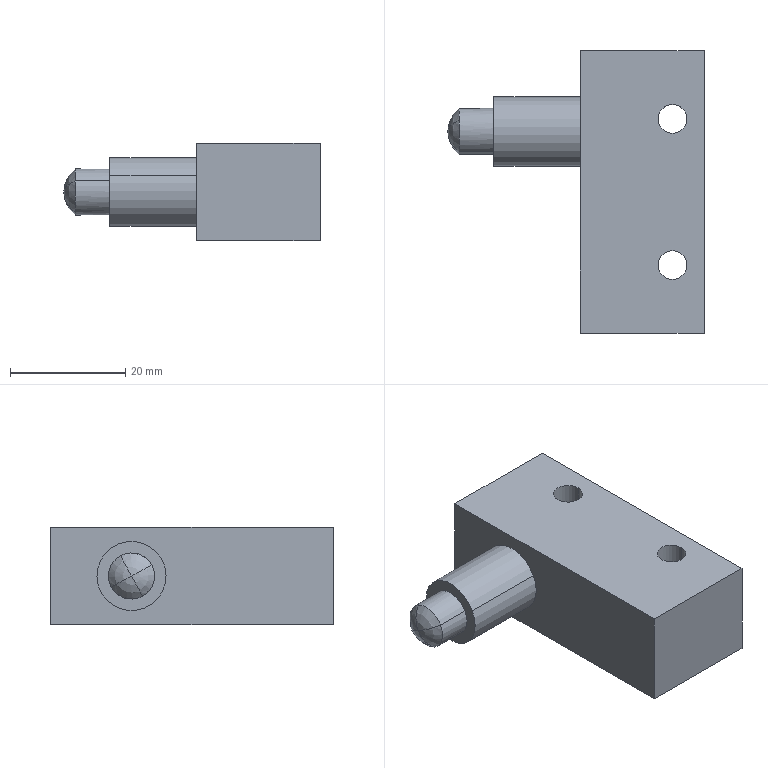Part | CATIA | 1 solid | 19 faces | box 44.5 x 49 x 17 mm | volume 19294 mm3 | cylinder 8 | plane 7 | sphere 4 | commonest cylinder face diameters 5 x4 8 x2 12 x2
STEP:
#1=CARTESIAN_POINT('',(-16.,17.935,11.377));
#2=VERTEX_POINT('',#1);
#3=CARTESIAN_POINT('',(-31.,17.935,11.377));
#4=VERTEX_POINT('',#3);
#5=CARTESIAN_POINT('',(-27.5,17.935,11.377));
#6=DIRECTION('',(-1.,0.,0.));
#7=VECTOR('',#6,1.);
#8=LINE('',#5,#7);
#9=EDGE_CURVE('',#2,#4,#8,.T.);
#10=ORIENTED_EDGE('',*,*,#9,.T.);
#11=CARTESIAN_POINT('',(-31.,28.465,5.623));
#12=VERTEX_POINT('',#11);
#13=CARTESIAN_POINT('',(-31.,23.2,8.5));
#14=DIRECTION('',(-1.,0.,0.));
#15=AXIS2_PLACEMENT_3D('',#13,#14,$);
#16=CIRCLE('',#15,6.);
#17=EDGE_CURVE('',#12,#4,#16,.T.);
#18=ORIENTED_EDGE('',*,*,#17,.F.);
#19=CARTESIAN_POINT('',(-16.,28.465,5.623));
#20=VERTEX_POINT('',#19);
#21=CARTESIAN_POINT('',(-27.5,28.465,5.623));
#22=DIRECTION('',(-1.,0.,0.));
#23=VECTOR('',#22,1.);
#24=LINE('',#21,#23);
#25=EDGE_CURVE('',#20,#12,#24,.T.);
#26=ORIENTED_EDGE('',*,*,#25,.F.);
#27=CARTESIAN_POINT('',(-16.,23.2,8.5));
#28=DIRECTION('',(-1.,0.,0.));
#29=AXIS2_PLACEMENT_3D('',#27,#28,$);
#30=CIRCLE('',#29,6.);
#31=EDGE_CURVE('',#20,#2,#30,.T.);
#32=ORIENTED_EDGE('',*,*,#31,.T.);
#33=EDGE_LOOP('',(#10,#18,#26,#32));
#34=FACE_OUTER_BOUND('',#33,.T.);
#35=CARTESIAN_POINT('',(-27.5,23.2,8.5));
#36=DIRECTION('',(-1.,0.,0.));
#37=DIRECTION('',(0.,0.8776,-0.4794));
#38=AXIS2_PLACEMENT_3D('',#35,#36,#37);
#39=CYLINDRICAL_SURFACE('',#38,6.);
#40=ADVANCED_FACE('',(#34),#39,.T.);
#41=ORIENTED_EDGE('',*,*,#25,.T.);
#42=CARTESIAN_POINT('',(-31.,23.2,8.5));
#43=DIRECTION('',(-1.,0.,0.));
#44=AXIS2_PLACEMENT_3D('',#42,#43,$);
#45=CIRCLE('',#44,6.);
#46=EDGE_CURVE('',#4,#12,#45,.T.);
#47=ORIENTED_EDGE('',*,*,#46,.F.);
#48=ORIENTED_EDGE('',*,*,#9,.F.);
#49=CARTESIAN_POINT('',(-16.,23.2,8.5));
#50=DIRECTION('',(-1.,0.,0.));
#51=AXIS2_PLACEMENT_3D('',#49,#50,$);
#52=CIRCLE('',#51,6.);
#53=EDGE_CURVE('',#2,#20,#52,.T.);
#54=ORIENTED_EDGE('',*,*,#53,.T.);
#55=EDGE_LOOP('',(#41,#47,#48,#54));
#56=FACE_OUTER_BOUND('',#55,.T.);
#57=CARTESIAN_POINT('',(-27.5,23.2,8.5));
#58=DIRECTION('',(-1.,0.,0.));
#59=DIRECTION('',(0.,-0.8776,0.4794));
#60=AXIS2_PLACEMENT_3D('',#57,#58,#59);
#61=CYLINDRICAL_SURFACE('',#60,6.);
#62=ADVANCED_FACE('',(#56),#61,.T.);
#63=ORIENTED_EDGE('',*,*,#46,.T.);
#64=ORIENTED_EDGE('',*,*,#17,.T.);
#65=EDGE_LOOP('',(#63,#64));
#66=FACE_OUTER_BOUND('',#65,.T.);
#67=CARTESIAN_POINT('',(-31.,26.71,6.582));
#68=VERTEX_POINT('',#67);
#69=CARTESIAN_POINT('',(-31.,19.69,10.418));
#70=VERTEX_POINT('',#69);
#71=CARTESIAN_POINT('',(-31.,23.2,8.5));
#72=DIRECTION('',(-1.,0.,0.));
#73=AXIS2_PLACEMENT_3D('',#71,#72,$);
#74=CIRCLE('',#73,4.);
#75=EDGE_CURVE('',#68,#70,#74,.T.);
#76=ORIENTED_EDGE('',*,*,#75,.F.);
#77=CARTESIAN_POINT('',(-31.,23.2,8.5));
#78=DIRECTION('',(-1.,0.,0.));
#79=AXIS2_PLACEMENT_3D('',#77,#78,$);
#80=CIRCLE('',#79,4.);
#81=EDGE_CURVE('',#70,#68,#80,.T.);
#82=ORIENTED_EDGE('',*,*,#81,.F.);
#83=EDGE_LOOP('',(#76,#82));
#84=FACE_BOUND('',#83,.T.);
#85=CARTESIAN_POINT('',(-31.,29.2,8.5));
#86=DIRECTION('',(-1.,0.,0.));
#87=DIRECTION('',(0.,1.,0.));
#88=AXIS2_PLACEMENT_3D('',#85,#86,#87);
#89=PLANE('',#88);
#90=ADVANCED_FACE('',(#66,#84),#89,.T.);
#91=CARTESIAN_POINT('',(-16.,37.2,0.));
#92=VERTEX_POINT('',#91);
#93=CARTESIAN_POINT('',(-16.,37.2,17.));
#94=VERTEX_POINT('',#93);
#95=CARTESIAN_POINT('',(-16.,37.2,8.5));
#96=DIRECTION('',(0.,0.,1.));
#97=VECTOR('',#96,1.);
#98=LINE('',#95,#97);
#99=EDGE_CURVE('',#92,#94,#98,.T.);
#100=ORIENTED_EDGE('',*,*,#99,.F.);
#101=CARTESIAN_POINT('',(-16.,-11.8,0.));
#102=VERTEX_POINT('',#101);
#103=CARTESIAN_POINT('',(-16.,12.7,0.));
#104=DIRECTION('',(0.,-1.,0.));
#105=VECTOR('',#104,1.);
#106=LINE('',#103,#105);
#107=EDGE_CURVE('',#92,#102,#106,.T.);
#108=ORIENTED_EDGE('',*,*,#107,.T.);
#109=CARTESIAN_POINT('',(-16.,-11.8,17.));
#110=VERTEX_POINT('',#109);
#111=CARTESIAN_POINT('',(-16.,-11.8,8.5));
#112=DIRECTION('',(0.,0.,1.));
#113=VECTOR('',#112,1.);
#114=LINE('',#111,#113);
#115=EDGE_CURVE('',#102,#110,#114,.T.);
#116=ORIENTED_EDGE('',*,*,#115,.T.);
#117=CARTESIAN_POINT('',(-16.,12.7,17.));
#118=DIRECTION('',(0.,-1.,0.));
#119=VECTOR('',#118,1.);
#120=LINE('',#117,#119);
#121=EDGE_CURVE('',#94,#110,#120,.T.);
#122=ORIENTED_EDGE('',*,*,#121,.F.);
#123=EDGE_LOOP('',(#100,#108,#116,#122));
#124=FACE_OUTER_BOUND('',#123,.T.);
#125=ORIENTED_EDGE('',*,*,#31,.F.);
#126=ORIENTED_EDGE('',*,*,#53,.F.);
#127=EDGE_LOOP('',(#125,#126));
#128=FACE_BOUND('',#127,.T.);
#129=CARTESIAN_POINT('',(-16.,37.2,0.));
#130=DIRECTION('',(-1.,0.,0.));
#131=DIRECTION('',(0.,-1.,0.));
#132=AXIS2_PLACEMENT_3D('',#129,#130,#131);
#133=PLANE('',#132);
#134=ADVANCED_FACE('',(#124,#128),#133,.T.);
#135=CARTESIAN_POINT('',(-37.,19.69,10.418));
#136=VERTEX_POINT('',#135);
#137=CARTESIAN_POINT('',(-27.5,19.69,10.418));
#138=DIRECTION('',(-1.,0.,0.));
#139=VECTOR('',#138,1.);
#140=LINE('',#137,#139);
#141=EDGE_CURVE('',#70,#136,#140,.T.);
#142=ORIENTED_EDGE('',*,*,#141,.T.);
#143=CARTESIAN_POINT('',(-37.,21.282,4.99));
#144=VERTEX_POINT('',#143);
#145=CARTESIAN_POINT('',(-37.,23.2,8.5));
#146=DIRECTION('',(-1.,0.,0.));
#147=AXIS2_PLACEMENT_3D('',#145,#146,$);
#148=CIRCLE('',#147,4.);
#149=EDGE_CURVE('',#144,#136,#148,.T.);
#150=ORIENTED_EDGE('',*,*,#149,.F.);
#151=CARTESIAN_POINT('',(-37.,26.71,6.582));
#152=VERTEX_POINT('',#151);
#153=CARTESIAN_POINT('',(-37.,23.2,8.5));
#154=DIRECTION('',(-1.,0.,0.));
#155=AXIS2_PLACEMENT_3D('',#153,#154,$);
#156=CIRCLE('',#155,4.);
#157=EDGE_CURVE('',#152,#144,#156,.T.);
#158=ORIENTED_EDGE('',*,*,#157,.F.);
#159=CARTESIAN_POINT('',(-27.5,26.71,6.582));
#160=DIRECTION('',(-1.,0.,0.));
#161=VECTOR('',#160,1.);
#162=LINE('',#159,#161);
#163=EDGE_CURVE('',#68,#152,#162,.T.);
#164=ORIENTED_EDGE('',*,*,#163,.F.);
#165=ORIENTED_EDGE('',*,*,#75,.T.);
#166=EDGE_LOOP('',(#142,#150,#158,#164,#165));
#167=FACE_OUTER_BOUND('',#166,.T.);
#168=CARTESIAN_POINT('',(-27.5,23.2,8.5));
#169=DIRECTION('',(-1.,0.,0.));
#170=DIRECTION('',(0.,0.8776,-0.4794));
#171=AXIS2_PLACEMENT_3D('',#168,#169,#170);
#172=CYLINDRICAL_SURFACE('',#171,4.);
#173=ADVANCED_FACE('',(#167),#172,.T.);
#174=ORIENTED_EDGE('',*,*,#163,.T.);
#175=CARTESIAN_POINT('',(-37.,25.118,12.01));
#176=VERTEX_POINT('',#175);
#177=CARTESIAN_POINT('',(-37.,23.2,8.5));
#178=DIRECTION('',(-1.,0.,0.));
#179=AXIS2_PLACEMENT_3D('',#177,#178,$);
#180=CIRCLE('',#179,4.);
#181=EDGE_CURVE('',#176,#152,#180,.T.);
#182=ORIENTED_EDGE('',*,*,#181,.F.);
#183=CARTESIAN_POINT('',(-37.,23.2,8.5));
#184=DIRECTION('',(-1.,0.,0.));
#185=AXIS2_PLACEMENT_3D('',#183,#184,$);
#186=CIRCLE('',#185,4.);
#187=EDGE_CURVE('',#136,#176,#186,.T.);
#188=ORIENTED_EDGE('',*,*,#187,.F.);
#189=ORIENTED_EDGE('',*,*,#141,.F.);
#190=ORIENTED_EDGE('',*,*,#81,.T.);
#191=EDGE_LOOP('',(#174,#182,#188,#189,#190));
#192=FACE_OUTER_BOUND('',#191,.T.);
#193=CARTESIAN_POINT('',(-27.5,23.2,8.5));
#194=DIRECTION('',(-1.,0.,0.));
#195=DIRECTION('',(0.,-0.8776,0.4794));
#196=AXIS2_PLACEMENT_3D('',#193,#194,#195);
#197=CYLINDRICAL_SURFACE('',#196,4.);
#198=ADVANCED_FACE('',(#192),#197,.T.);
#199=CARTESIAN_POINT('',(5.5,37.2,0.));
#200=VERTEX_POINT('',#199);
#201=CARTESIAN_POINT('',(5.5,37.2,17.));
#202=VERTEX_POINT('',#201);
#203=CARTESIAN_POINT('',(5.5,37.2,8.5));
#204=DIRECTION('',(0.,0.,1.));
#205=VECTOR('',#204,1.);
#206=LINE('',#203,#205);
#207=EDGE_CURVE('',#200,#202,#206,.T.);
#208=ORIENTED_EDGE('',*,*,#207,.F.);
#209=CARTESIAN_POINT('',(-5.25,37.2,0.));
#210=DIRECTION('',(1.,0.,0.));
#211=VECTOR('',#210,1.);
#212=LINE('',#209,#211);
#213=EDGE_CURVE('',#200,#92,#212,.F.);
#214=ORIENTED_EDGE('',*,*,#213,.T.);
#215=ORIENTED_EDGE('',*,*,#99,.T.);
#216=CARTESIAN_POINT('',(-5.25,37.2,17.));
#217=DIRECTION('',(1.,0.,0.));
#218=VECTOR('',#217,1.);
#219=LINE('',#216,#218);
#220=EDGE_CURVE('',#202,#94,#219,.F.);
#221=ORIENTED_EDGE('',*,*,#220,.F.);
#222=EDGE_LOOP('',(#208,#214,#215,#221));
#223=FACE_OUTER_BOUND('',#222,.T.);
#224=CARTESIAN_POINT('',(-16.,37.2,0.));
#225=DIRECTION('',(0.,-1.,0.));
#226=DIRECTION('',(1.,0.,0.));
#227=AXIS2_PLACEMENT_3D('',#224,#225,#226);
#228=PLANE('',#227);
#229=ADVANCED_FACE('',(#223),#228,.F.);
#230=ORIENTED_EDGE('',*,*,#213,.F.);
#231=CARTESIAN_POINT('',(5.5,-11.8,0.));
#232=VERTEX_POINT('',#231);
#233=CARTESIAN_POINT('',(5.5,12.7,0.));
#234=DIRECTION('',(0.,1.,0.));
#235=VECTOR('',#234,1.);
#236=LINE('',#233,#235);
#237=EDGE_CURVE('',#232,#200,#236,.T.);
#238=ORIENTED_EDGE('',*,*,#237,.F.);
#239=CARTESIAN_POINT('',(-5.25,-11.8,0.));
#240=DIRECTION('',(-1.,0.,0.));
#241=VECTOR('',#240,1.);
#242=LINE('',#239,#241);
#243=EDGE_CURVE('',#102,#232,#242,.F.);
#244=ORIENTED_EDGE('',*,*,#243,.F.);
#245=ORIENTED_EDGE('',*,*,#107,.F.);
#246=EDGE_LOOP('',(#230,#238,#244,#245));
#247=FACE_OUTER_BOUND('',#246,.T.);
#248=CARTESIAN_POINT('',(2.5,25.4,0.));
#249=VERTEX_POINT('',#248);
#250=CARTESIAN_POINT('',(-2.5,25.4,0.));
#251=VERTEX_POINT('',#250);
#252=CARTESIAN_POINT('',(0.,25.4,0.));
#253=DIRECTION('',(0.,0.,1.));
#254=AXIS2_PLACEMENT_3D('',#252,#253,$);
#255=CIRCLE('',#254,2.5);
#256=EDGE_CURVE('',#249,#251,#255,.T.);
#257=ORIENTED_EDGE('',*,*,#256,.T.);
#258=CARTESIAN_POINT('',(0.,25.4,0.));
#259=DIRECTION('',(0.,0.,1.));
#260=AXIS2_PLACEMENT_3D('',#258,#259,$);
#261=CIRCLE('',#260,2.5);
#262=EDGE_CURVE('',#251,#249,#261,.T.);
#263=ORIENTED_EDGE('',*,*,#262,.T.);
#264=EDGE_LOOP('',(#257,#263));
#265=FACE_BOUND('',#264,.T.);
#266=CARTESIAN_POINT('',(2.5,0.,0.));
#267=VERTEX_POINT('',#266);
#268=CARTESIAN_POINT('',(-2.5,0.,0.));
#269=VERTEX_POINT('',#268);
#270=CARTESIAN_POINT('',(0.,0.,0.));
#271=DIRECTION('',(0.,0.,1.));
#272=AXIS2_PLACEMENT_3D('',#270,#271,$);
#273=CIRCLE('',#272,2.5);
#274=EDGE_CURVE('',#267,#269,#273,.T.);
#275=ORIENTED_EDGE('',*,*,#274,.T.);
#276=CARTESIAN_POINT('',(0.,0.,0.));
#277=DIRECTION('',(0.,0.,1.));
#278=AXIS2_PLACEMENT_3D('',#276,#277,$);
#279=CIRCLE('',#278,2.5);
#280=EDGE_CURVE('',#269,#267,#279,.T.);
#281=ORIENTED_EDGE('',*,*,#280,.T.);
#282=EDGE_LOOP('',(#275,#281));
#283=FACE_BOUND('',#282,.T.);
#284=CARTESIAN_POINT('',(0.,0.,0.));
#285=DIRECTION('',(0.,0.,1.));
#286=DIRECTION('',(1.,0.,0.));
#287=AXIS2_PLACEMENT_3D('',#284,#285,#286);
#288=PLANE('',#287);
#289=ADVANCED_FACE('',(#247,#265,#283),#288,.F.);
#290=ORIENTED_EDGE('',*,*,#115,.F.);
#291=ORIENTED_EDGE('',*,*,#243,.T.);
#292=CARTESIAN_POINT('',(5.5,-11.8,17.));
#293=VERTEX_POINT('',#292);
#294=CARTESIAN_POINT('',(5.5,-11.8,8.5));
#295=DIRECTION('',(0.,0.,1.));
#296=VECTOR('',#295,1.);
#297=LINE('',#294,#296);
#298=EDGE_CURVE('',#232,#293,#297,.T.);
#299=ORIENTED_EDGE('',*,*,#298,.T.);
#300=CARTESIAN_POINT('',(-5.25,-11.8,17.));
#301=DIRECTION('',(-1.,0.,0.));
#302=VECTOR('',#301,1.);
#303=LINE('',#300,#302);
#304=EDGE_CURVE('',#110,#293,#303,.F.);
#305=ORIENTED_EDGE('',*,*,#304,.F.);
#306=EDGE_LOOP('',(#290,#291,#299,#305));
#307=FACE_OUTER_BOUND('',#306,.T.);
#308=CARTESIAN_POINT('',(5.5,-11.8,0.));
#309=DIRECTION('',(0.,1.,0.));
#310=DIRECTION('',(-1.,0.,0.));
#311=AXIS2_PLACEMENT_3D('',#308,#309,#310);
#312=PLANE('',#311);
#313=ADVANCED_FACE('',(#307),#312,.F.);
#314=ORIENTED_EDGE('',*,*,#121,.T.);
#315=ORIENTED_EDGE('',*,*,#304,.T.);
#316=CARTESIAN_POINT('',(5.5,12.7,17.));
#317=DIRECTION('',(0.,1.,0.));
#318=VECTOR('',#317,1.);
#319=LINE('',#316,#318);
#320=EDGE_CURVE('',#293,#202,#319,.T.);
#321=ORIENTED_EDGE('',*,*,#320,.T.);
#322=ORIENTED_EDGE('',*,*,#220,.T.);
#323=EDGE_LOOP('',(#314,#315,#321,#322));
#324=FACE_OUTER_BOUND('',#323,.T.);
#325=CARTESIAN_POINT('',(2.5,25.4,17.));
#326=VERTEX_POINT('',#325);
#327=CARTESIAN_POINT('',(-2.5,25.4,17.));
#328=VERTEX_POINT('',#327);
#329=CARTESIAN_POINT('',(0.,25.4,17.));
#330=DIRECTION('',(0.,0.,1.));
#331=AXIS2_PLACEMENT_3D('',#329,#330,$);
#332=CIRCLE('',#331,2.5);
#333=EDGE_CURVE('',#326,#328,#332,.T.);
#334=ORIENTED_EDGE('',*,*,#333,.F.);
#335=CARTESIAN_POINT('',(0.,25.4,17.));
#336=DIRECTION('',(0.,0.,1.));
#337=AXIS2_PLACEMENT_3D('',#335,#336,$);
#338=CIRCLE('',#337,2.5);
#339=EDGE_CURVE('',#328,#326,#338,.T.);
#340=ORIENTED_EDGE('',*,*,#339,.F.);
#341=EDGE_LOOP('',(#334,#340));
#342=FACE_BOUND('',#341,.T.);
#343=CARTESIAN_POINT('',(2.5,0.,17.));
#344=VERTEX_POINT('',#343);
#345=CARTESIAN_POINT('',(-2.5,0.,17.));
#346=VERTEX_POINT('',#345);
#347=CARTESIAN_POINT('',(0.,0.,17.));
#348=DIRECTION('',(0.,0.,1.));
#349=AXIS2_PLACEMENT_3D('',#347,#348,$);
#350=CIRCLE('',#349,2.5);
#351=EDGE_CURVE('',#344,#346,#350,.T.);
#352=ORIENTED_EDGE('',*,*,#351,.F.);
#353=CARTESIAN_POINT('',(0.,0.,17.));
#354=DIRECTION('',(0.,0.,1.));
#355=AXIS2_PLACEMENT_3D('',#353,#354,$);
#356=CIRCLE('',#355,2.5);
#357=EDGE_CURVE('',#346,#344,#356,.T.);
#358=ORIENTED_EDGE('',*,*,#357,.F.);
#359=EDGE_LOOP('',(#352,#358));
#360=FACE_BOUND('',#359,.T.);
#361=CARTESIAN_POINT('',(0.,0.,17.));
#362=DIRECTION('',(0.,0.,1.));
#363=DIRECTION('',(1.,0.,0.));
#364=AXIS2_PLACEMENT_3D('',#361,#362,#363);
#365=PLANE('',#364);
#366=ADVANCED_FACE('',(#324,#342,#360),#365,.T.);
#367=CARTESIAN_POINT('',(-39.,23.2,8.5));
#368=VERTEX_POINT('',#367);
#369=CARTESIAN_POINT('',(-34.,23.2,8.5));
#370=DIRECTION('',(0.,0.8776,-0.4794));
#371=AXIS2_PLACEMENT_3D('',#369,#370,$);
#372=CIRCLE('',#371,5.);
#373=EDGE_CURVE('',#144,#368,#372,.T.);
#374=ORIENTED_EDGE('',*,*,#373,.F.);
#375=ORIENTED_EDGE('',*,*,#149,.T.);
#376=CARTESIAN_POINT('',(-34.,23.2,8.5));
#377=DIRECTION('',(0.,-0.4794,-0.8776));
#378=AXIS2_PLACEMENT_3D('',#376,#377,$);
#379=CIRCLE('',#378,5.);
#380=EDGE_CURVE('',#136,#368,#379,.T.);
#381=ORIENTED_EDGE('',*,*,#380,.T.);
#382=EDGE_LOOP('',(#374,#375,#381));
#383=FACE_OUTER_BOUND('',#382,.T.);
#384=CARTESIAN_POINT('',(-34.,23.2,8.5));
#385=DIRECTION('',(-1.,0.,0.));
#386=DIRECTION('',(0.,-0.4794,-0.8776));
#387=AXIS2_PLACEMENT_3D('',#384,#385,#386);
#388=SPHERICAL_SURFACE('',#387,5.);
#389=ADVANCED_FACE('',(#383),#388,.T.);
#390=ORIENTED_EDGE('',*,*,#373,.T.);
#391=CARTESIAN_POINT('',(-34.,23.2,8.5));
#392=DIRECTION('',(0.,0.4794,0.8776));
#393=AXIS2_PLACEMENT_3D('',#391,#392,$);
#394=CIRCLE('',#393,5.);
#395=EDGE_CURVE('',#152,#368,#394,.T.);
#396=ORIENTED_EDGE('',*,*,#395,.F.);
#397=ORIENTED_EDGE('',*,*,#157,.T.);
#398=EDGE_LOOP('',(#390,#396,#397));
#399=FACE_OUTER_BOUND('',#398,.T.);
#400=CARTESIAN_POINT('',(-34.,23.2,8.5));
#401=DIRECTION('',(-1.,0.,0.));
#402=DIRECTION('',(0.,0.8776,-0.4794));
#403=AXIS2_PLACEMENT_3D('',#400,#401,#402);
#404=SPHERICAL_SURFACE('',#403,5.);
#405=ADVANCED_FACE('',(#399),#404,.T.);
#406=CARTESIAN_POINT('',(-34.,23.2,8.5));
#407=DIRECTION('',(0.,-0.8776,0.4794));
#408=AXIS2_PLACEMENT_3D('',#406,#407,$);
#409=CIRCLE('',#408,5.);
#410=EDGE_CURVE('',#176,#368,#409,.T.);
#411=ORIENTED_EDGE('',*,*,#410,.F.);
#412=ORIENTED_EDGE('',*,*,#181,.T.);
#413=ORIENTED_EDGE('',*,*,#395,.T.);
#414=EDGE_LOOP('',(#411,#412,#413));
#415=FACE_OUTER_BOUND('',#414,.T.);
#416=CARTESIAN_POINT('',(-34.,23.2,8.5));
#417=DIRECTION('',(-1.,0.,0.));
#418=DIRECTION('',(0.,0.4794,0.8776));
#419=AXIS2_PLACEMENT_3D('',#416,#417,#418);
#420=SPHERICAL_SURFACE('',#419,5.);
#421=ADVANCED_FACE('',(#415),#420,.T.);
#422=ORIENTED_EDGE('',*,*,#410,.T.);
#423=ORIENTED_EDGE('',*,*,#380,.F.);
#424=ORIENTED_EDGE('',*,*,#187,.T.);
#425=EDGE_LOOP('',(#422,#423,#424));
#426=FACE_OUTER_BOUND('',#425,.T.);
#427=CARTESIAN_POINT('',(-34.,23.2,8.5));
#428=DIRECTION('',(-1.,0.,0.));
#429=DIRECTION('',(0.,-0.8776,0.4794));
#430=AXIS2_PLACEMENT_3D('',#427,#428,#429);
#431=SPHERICAL_SURFACE('',#430,5.);
#432=ADVANCED_FACE('',(#426),#431,.T.);
#433=ORIENTED_EDGE('',*,*,#298,.F.);
#434=ORIENTED_EDGE('',*,*,#237,.T.);
#435=ORIENTED_EDGE('',*,*,#207,.T.);
#436=ORIENTED_EDGE('',*,*,#320,.F.);
#437=EDGE_LOOP('',(#433,#434,#435,#436));
#438=FACE_OUTER_BOUND('',#437,.T.);
#439=CARTESIAN_POINT('',(5.5,-11.8,0.));
#440=DIRECTION('',(1.,0.,0.));
#441=DIRECTION('',(0.,1.,0.));
#442=AXIS2_PLACEMENT_3D('',#439,#440,#441);
#443=PLANE('',#442);
#444=ADVANCED_FACE('',(#438),#443,.T.);
#445=ORIENTED_EDGE('',*,*,#256,.F.);
#446=CARTESIAN_POINT('',(2.5,25.4,7.89));
#447=DIRECTION('',(0.,0.,1.));
#448=VECTOR('',#447,1.);
#449=LINE('',#446,#448);
#450=EDGE_CURVE('',#326,#249,#449,.F.);
#451=ORIENTED_EDGE('',*,*,#450,.F.);
#452=ORIENTED_EDGE('',*,*,#333,.T.);
#453=CARTESIAN_POINT('',(-2.5,25.4,7.89));
#454=DIRECTION('',(0.,0.,1.));
#455=VECTOR('',#454,1.);
#456=LINE('',#453,#455);
#457=EDGE_CURVE('',#328,#251,#456,.F.);
#458=ORIENTED_EDGE('',*,*,#457,.T.);
#459=EDGE_LOOP('',(#445,#451,#452,#458));
#460=FACE_OUTER_BOUND('',#459,.T.);
#461=CARTESIAN_POINT('',(0.,25.4,7.89));
#462=DIRECTION('',(0.,0.,1.));
#463=DIRECTION('',(1.,0.,0.));
#464=AXIS2_PLACEMENT_3D('',#461,#462,#463);
#465=CYLINDRICAL_SURFACE('',#464,2.5);
#466=ADVANCED_FACE('',(#460),#465,.F.);
#467=ORIENTED_EDGE('',*,*,#262,.F.);
#468=ORIENTED_EDGE('',*,*,#457,.F.);
#469=ORIENTED_EDGE('',*,*,#339,.T.);
#470=ORIENTED_EDGE('',*,*,#450,.T.);
#471=EDGE_LOOP('',(#467,#468,#469,#470));
#472=FACE_OUTER_BOUND('',#471,.T.);
#473=CARTESIAN_POINT('',(0.,25.4,7.89));
#474=DIRECTION('',(0.,0.,1.));
#475=DIRECTION('',(-1.,0.,0.));
#476=AXIS2_PLACEMENT_3D('',#473,#474,#475);
#477=CYLINDRICAL_SURFACE('',#476,2.5);
#478=ADVANCED_FACE('',(#472),#477,.F.);
#479=ORIENTED_EDGE('',*,*,#274,.F.);
#480=CARTESIAN_POINT('',(2.5,0.,7.89));
#481=DIRECTION('',(0.,0.,1.));
#482=VECTOR('',#481,1.);
#483=LINE('',#480,#482);
#484=EDGE_CURVE('',#344,#267,#483,.F.);
#485=ORIENTED_EDGE('',*,*,#484,.F.);
#486=ORIENTED_EDGE('',*,*,#351,.T.);
#487=CARTESIAN_POINT('',(-2.5,0.,7.89));
#488=DIRECTION('',(0.,0.,1.));
#489=VECTOR('',#488,1.);
#490=LINE('',#487,#489);
#491=EDGE_CURVE('',#346,#269,#490,.F.);
#492=ORIENTED_EDGE('',*,*,#491,.T.);
#493=EDGE_LOOP('',(#479,#485,#486,#492));
#494=FACE_OUTER_BOUND('',#493,.T.);
#495=CARTESIAN_POINT('',(0.,0.,7.89));
#496=DIRECTION('',(0.,0.,1.));
#497=DIRECTION('',(1.,0.,0.));
#498=AXIS2_PLACEMENT_3D('',#495,#496,#497);
#499=CYLINDRICAL_SURFACE('',#498,2.5);
#500=ADVANCED_FACE('',(#494),#499,.F.);
#501=ORIENTED_EDGE('',*,*,#280,.F.);
#502=ORIENTED_EDGE('',*,*,#491,.F.);
#503=ORIENTED_EDGE('',*,*,#357,.T.);
#504=ORIENTED_EDGE('',*,*,#484,.T.);
#505=EDGE_LOOP('',(#501,#502,#503,#504));
#506=FACE_OUTER_BOUND('',#505,.T.);
#507=CARTESIAN_POINT('',(0.,0.,7.89));
#508=DIRECTION('',(0.,0.,1.));
#509=DIRECTION('',(-1.,0.,0.));
#510=AXIS2_PLACEMENT_3D('',#507,#508,#509);
#511=CYLINDRICAL_SURFACE('',#510,2.5);
#512=ADVANCED_FACE('',(#506),#511,.F.);
#513=CLOSED_SHELL('',(#40,#62,#90,#134,#173,#198,#229,#289,#313,#366,#389,#405,#421,#432,#444,#466,#478,#500,#512));
#514=MANIFOLD_SOLID_BREP('',#513);
#515=(LENGTH_UNIT()NAMED_UNIT(*)SI_UNIT(.MILLI.,.METRE.));
#516=UNCERTAINTY_MEASURE_WITH_UNIT(LENGTH_MEASURE(0.005),#515,'','');
#517=(NAMED_UNIT(*)PLANE_ANGLE_UNIT()SI_UNIT($,.RADIAN.));
#518=(NAMED_UNIT(*)SI_UNIT($,.STERADIAN.)SOLID_ANGLE_UNIT());
#519=(GEOMETRIC_REPRESENTATION_CONTEXT(3)GLOBAL_UNCERTAINTY_ASSIGNED_CONTEXT((#516))GLOBAL_UNIT_ASSIGNED_CONTEXT((#515,#517,#518))REPRESENTATION_CONTEXT('',''));
#520=ADVANCED_BREP_SHAPE_REPRESENTATION('',(#514),#519);